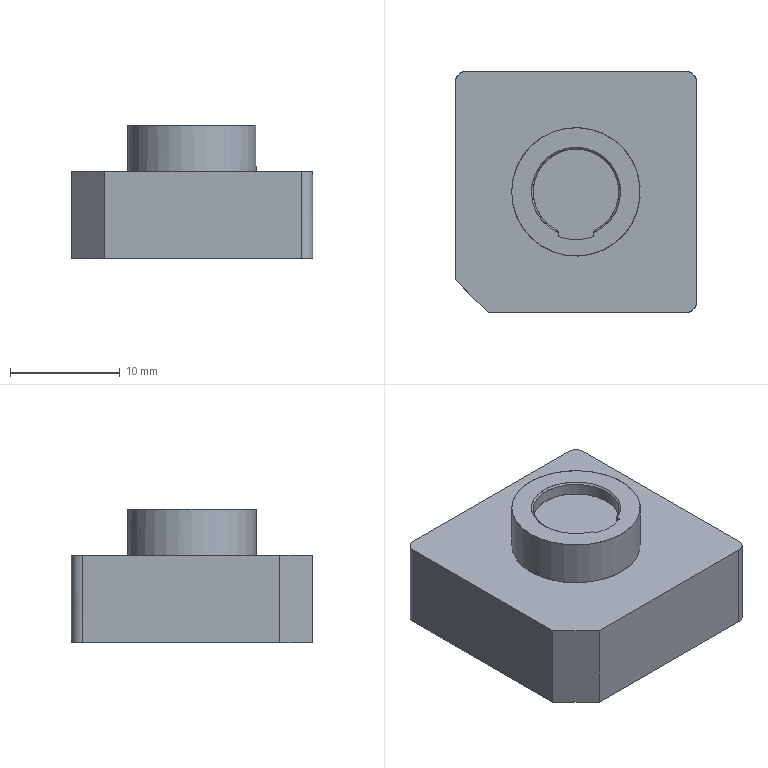NC program | PowerMill | posted by the shop | part box 22 x 22 x 12.219 mm
Lines 1 to 2304 of 55612, first 2083 of 2303 lines:
%
G40 G49 G17 G80
( TOOL ID   D10C_1_1 )
( TOOL DIA. 10. TIP RAD 0 LENGTH 67.68 )
( Z = -.071 )
T1 M6
T15
G91 G28 Z0
G0 G90 G54
M08
S8000 M3
G0 X0 Y0 M8
G43 Z10.2 H1
X13.78 Y13.78
Z1.129
G1 Z-.071 F6000
X-13.78 F10000
Y8.268
X13.78
Y2.756
X-13.78
Y-2.756
X13.78
Y-8.268
X-13.78
Y-13.78
X13.78
X18.78
G0 Z10.2
X0 Y0
Z9.879
X19.055 Y5.589
Z.705
G1 Z-.495 F6000
X18.528 F10000
G3 X13.78 Y.842 I0 J-4.748
G1 Y-12.78
G2 X12.78 Y-13.78 I-1. J0
G1 X-12.78
G2 X-13.78 Y-12.78 I0 J1.
G1 Y12.78
G2 X-12.78 Y13.78 I1. J0
G1 X12.78
G2 X13.78 Y12.78 I0 J-1.
G1 Y.842
X11.106 Y.677
X11.124 Y.387
Y-.387
X11.076 Y-1.16
X10.962 Y-1.934
X10.796 Y-2.707
X10.579 Y-3.48
X10.441 Y-3.857
X9.93 Y-5.027
X9.507 Y-5.801
X8.894 Y-6.698
X8.369 Y-7.348
X7.348 Y-8.369
X6.698 Y-8.894
X5.801 Y-9.507
X5.027 Y-9.93
X3.857 Y-10.441
X3.48 Y-10.579
X2.707 Y-10.796
X1.934 Y-10.962
X1.16 Y-11.076
X.387 Y-11.124
X-.387
X-1.16 Y-11.076
X-1.934 Y-10.962
X-2.707 Y-10.796
X-3.48 Y-10.579
X-3.857 Y-10.441
X-5.027 Y-9.93
X-5.801 Y-9.507
X-6.698 Y-8.894
X-7.348 Y-8.369
X-8.369 Y-7.348
X-8.894 Y-6.698
X-9.507 Y-5.801
X-9.93 Y-5.027
X-10.284 Y-4.254
X-10.579 Y-3.48
X-10.796 Y-2.707
X-10.962 Y-1.934
X-11.076 Y-1.16
X-11.124 Y-.387
Y.387
X-11.076 Y1.16
X-10.962 Y1.934
X-10.796 Y2.707
X-10.579 Y3.48
X-10.441 Y3.857
X-9.93 Y5.027
X-9.507 Y5.801
X-8.894 Y6.698
X-8.369 Y7.348
X-7.348 Y8.369
X-6.698 Y8.894
X-5.801 Y9.507
X-5.027 Y9.93
X-4.254 Y10.284
X-3.48 Y10.579
X-2.707 Y10.796
X-1.934 Y10.962
X-1.16 Y11.076
X-.387 Y11.124
X.387
X1.16 Y11.076
X1.934 Y10.962
X2.707 Y10.796
X3.48 Y10.579
X3.857 Y10.441
X5.027 Y9.93
X5.801 Y9.507
X6.698 Y8.894
X7.348 Y8.369
X8.369 Y7.348
X8.894 Y6.698
X9.507 Y5.801
X9.93 Y5.027
X10.284 Y4.254
X10.579 Y3.48
X10.796 Y2.707
X10.962 Y1.934
X11.076 Y1.16
X11.106 Y.677
X13.78 Y.842
G0 Z3.332
G1 X19.055 Y5.589
G0 Z.332
G1 Z-.868 F6000
X18.528 F10000
G3 X13.78 Y.842 I0 J-4.748
G1 Y-12.78
G2 X12.78 Y-13.78 I-1. J0
G1 X-12.78
G2 X-13.78 Y-12.78 I0 J1.
G1 Y12.78
G2 X-12.78 Y13.78 I1. J0
G1 X12.78
G2 X13.78 Y12.78 I0 J-1.
G1 Y.842
X11.106 Y.677
X11.124 Y.387
Y-.387
X11.076 Y-1.16
X10.962 Y-1.934
X10.796 Y-2.707
X10.579 Y-3.48
X10.441 Y-3.857
X9.93 Y-5.027
X9.507 Y-5.801
X8.894 Y-6.698
X8.369 Y-7.348
X7.348 Y-8.369
X6.698 Y-8.894
X5.801 Y-9.507
X5.027 Y-9.93
X3.857 Y-10.441
X3.48 Y-10.579
X2.707 Y-10.796
X1.934 Y-10.962
X1.16 Y-11.076
X.387 Y-11.124
X-.387
X-1.16 Y-11.076
X-1.934 Y-10.962
X-2.707 Y-10.796
X-3.48 Y-10.579
X-3.857 Y-10.441
X-5.027 Y-9.93
X-5.801 Y-9.507
X-6.698 Y-8.894
X-7.348 Y-8.369
X-8.369 Y-7.348
X-8.894 Y-6.698
X-9.507 Y-5.801
X-9.93 Y-5.027
X-10.284 Y-4.254
X-10.579 Y-3.48
X-10.796 Y-2.707
X-10.962 Y-1.934
X-11.076 Y-1.16
X-11.124 Y-.387
Y.387
X-11.076 Y1.16
X-10.962 Y1.934
X-10.796 Y2.707
X-10.579 Y3.48
X-10.441 Y3.857
X-9.93 Y5.027
X-9.507 Y5.801
X-8.894 Y6.698
X-8.369 Y7.348
X-7.348 Y8.369
X-6.698 Y8.894
X-5.801 Y9.507
X-5.027 Y9.93
X-4.254 Y10.284
X-3.48 Y10.579
X-2.707 Y10.796
X-1.934 Y10.962
X-1.16 Y11.076
X-.387 Y11.124
X.387
X1.16 Y11.076
X1.934 Y10.962
X2.707 Y10.796
X3.48 Y10.579
X3.857 Y10.441
X5.027 Y9.93
X5.801 Y9.507
X6.698 Y8.894
X7.348 Y8.369
X8.369 Y7.348
X8.894 Y6.698
X9.507 Y5.801
X9.93 Y5.027
X10.284 Y4.254
X10.579 Y3.48
X10.796 Y2.707
X10.962 Y1.934
X11.076 Y1.16
X11.106 Y.677
X13.78 Y.842
G0 Z2.958
G1 X19.055 Y5.589
G0 Z-.042
G1 Z-1.242 F6000
X18.528 F10000
G3 X13.78 Y.842 I0 J-4.748
G1 Y-12.78
G2 X12.78 Y-13.78 I-1. J0
G1 X-12.78
G2 X-13.78 Y-12.78 I0 J1.
G1 Y12.78
G2 X-12.78 Y13.78 I1. J0
G1 X12.78
G2 X13.78 Y12.78 I0 J-1.
G1 Y.842
X11.106 Y.677
X11.124 Y.387
Y-.387
X11.076 Y-1.16
X10.962 Y-1.934
X10.796 Y-2.707
X10.579 Y-3.48
X10.441 Y-3.857
X9.93 Y-5.027
X9.507 Y-5.801
X8.894 Y-6.698
X8.369 Y-7.348
X7.348 Y-8.369
X6.698 Y-8.894
X5.801 Y-9.507
X5.027 Y-9.93
X3.857 Y-10.441
X3.48 Y-10.579
X2.707 Y-10.796
X1.934 Y-10.962
X1.16 Y-11.076
X.387 Y-11.124
X-.387
X-1.16 Y-11.076
X-1.934 Y-10.962
X-2.707 Y-10.796
X-3.48 Y-10.579
X-3.857 Y-10.441
X-5.027 Y-9.93
X-5.801 Y-9.507
X-6.698 Y-8.894
X-7.348 Y-8.369
X-8.369 Y-7.348
X-8.894 Y-6.698
X-9.507 Y-5.801
X-9.93 Y-5.027
X-10.284 Y-4.254
X-10.579 Y-3.48
X-10.796 Y-2.707
X-10.962 Y-1.934
X-11.076 Y-1.16
X-11.124 Y-.387
Y.387
X-11.076 Y1.16
X-10.962 Y1.934
X-10.796 Y2.707
X-10.579 Y3.48
X-10.441 Y3.857
X-9.93 Y5.027
X-9.507 Y5.801
X-8.894 Y6.698
X-8.369 Y7.348
X-7.348 Y8.369
X-6.698 Y8.894
X-5.801 Y9.507
X-5.027 Y9.93
X-4.254 Y10.284
X-3.48 Y10.579
X-2.707 Y10.796
X-1.934 Y10.962
X-1.16 Y11.076
X-.387 Y11.124
X.387
X1.16 Y11.076
X1.934 Y10.962
X2.707 Y10.796
X3.48 Y10.579
X3.857 Y10.441
X5.027 Y9.93
X5.801 Y9.507
X6.698 Y8.894
X7.348 Y8.369
X8.369 Y7.348
X8.894 Y6.698
X9.507 Y5.801
X9.93 Y5.027
X10.284 Y4.254
X10.579 Y3.48
X10.796 Y2.707
X10.962 Y1.934
X11.076 Y1.16
X11.106 Y.677
X13.78 Y.842
G0 Z2.585
G1 X19.055 Y5.589
G0 Z-.415
G1 Z-1.615 F6000
X18.528 F10000
G3 X13.78 Y.842 I0 J-4.748
G1 Y-12.78
G2 X12.78 Y-13.78 I-1. J0
G1 X-12.78
G2 X-13.78 Y-12.78 I0 J1.
G1 Y12.78
G2 X-12.78 Y13.78 I1. J0
G1 X12.78
G2 X13.78 Y12.78 I0 J-1.
G1 Y.842
X11.106 Y.677
X11.124 Y.387
Y-.387
X11.076 Y-1.16
X10.962 Y-1.934
X10.796 Y-2.707
X10.579 Y-3.48
X10.441 Y-3.857
X9.93 Y-5.027
X9.507 Y-5.801
X8.894 Y-6.698
X8.369 Y-7.348
X7.348 Y-8.369
X6.698 Y-8.894
X5.801 Y-9.507
X5.027 Y-9.93
X3.857 Y-10.441
X3.48 Y-10.579
X2.707 Y-10.796
X1.934 Y-10.962
X1.16 Y-11.076
X.387 Y-11.124
X-.387
X-1.16 Y-11.076
X-1.934 Y-10.962
X-2.707 Y-10.796
X-3.48 Y-10.579
X-3.857 Y-10.441
X-5.027 Y-9.93
X-5.801 Y-9.507
X-6.698 Y-8.894
X-7.348 Y-8.369
X-8.369 Y-7.348
X-8.894 Y-6.698
X-9.507 Y-5.801
X-9.93 Y-5.027
X-10.284 Y-4.254
X-10.579 Y-3.48
X-10.796 Y-2.707
X-10.962 Y-1.934
X-11.076 Y-1.16
X-11.124 Y-.387
Y.387
X-11.076 Y1.16
X-10.962 Y1.934
X-10.796 Y2.707
X-10.579 Y3.48
X-10.441 Y3.857
X-9.93 Y5.027
X-9.507 Y5.801
X-8.894 Y6.698
X-8.369 Y7.348
X-7.348 Y8.369
X-6.698 Y8.894
X-5.801 Y9.507
X-5.027 Y9.93
X-4.254 Y10.284
X-3.48 Y10.579
X-2.707 Y10.796
X-1.934 Y10.962
X-1.16 Y11.076
X-.387 Y11.124
X.387
X1.16 Y11.076
X1.934 Y10.962
X2.707 Y10.796
X3.48 Y10.579
X3.857 Y10.441
X5.027 Y9.93
X5.801 Y9.507
X6.698 Y8.894
X7.348 Y8.369
X8.369 Y7.348
X8.894 Y6.698
X9.507 Y5.801
X9.93 Y5.027
X10.284 Y4.254
X10.579 Y3.48
X10.796 Y2.707
X10.962 Y1.934
X11.076 Y1.16
X11.106 Y.677
X13.78 Y.842
G0 Z2.211
G1 X19.055 Y5.589
G0 Z-.789
G1 Z-1.989 F6000
X18.528 F10000
G3 X13.78 Y.842 I0 J-4.748
G1 Y-12.78
G2 X12.78 Y-13.78 I-1. J0
G1 X-12.78
G2 X-13.78 Y-12.78 I0 J1.
G1 Y12.78
G2 X-12.78 Y13.78 I1. J0
G1 X12.78
G2 X13.78 Y12.78 I0 J-1.
G1 Y.842
X11.106 Y.677
X11.124 Y.387
Y-.387
X11.076 Y-1.16
X10.962 Y-1.934
X10.796 Y-2.707
X10.579 Y-3.48
X10.441 Y-3.857
X9.93 Y-5.027
X9.507 Y-5.801
X8.894 Y-6.698
X8.369 Y-7.348
X7.348 Y-8.369
X6.698 Y-8.894
X5.801 Y-9.507
X5.027 Y-9.93
X3.857 Y-10.441
X3.48 Y-10.579
X2.707 Y-10.796
X1.934 Y-10.962
X1.16 Y-11.076
X.387 Y-11.124
X-.387
X-1.16 Y-11.076
X-1.934 Y-10.962
X-2.707 Y-10.796
X-3.48 Y-10.579
X-3.857 Y-10.441
X-5.027 Y-9.93
X-5.801 Y-9.507
X-6.698 Y-8.894
X-7.348 Y-8.369
X-8.369 Y-7.348
X-8.894 Y-6.698
X-9.507 Y-5.801
X-9.93 Y-5.027
X-10.284 Y-4.254
X-10.579 Y-3.48
X-10.796 Y-2.707
X-10.962 Y-1.934
X-11.076 Y-1.16
X-11.124 Y-.387
Y.387
X-11.076 Y1.16
X-10.962 Y1.934
X-10.796 Y2.707
X-10.579 Y3.48
X-10.441 Y3.857
X-9.93 Y5.027
X-9.507 Y5.801
X-8.894 Y6.698
X-8.369 Y7.348
X-7.348 Y8.369
X-6.698 Y8.894
X-5.801 Y9.507
X-5.027 Y9.93
X-4.254 Y10.284
X-3.48 Y10.579
X-2.707 Y10.796
X-1.934 Y10.962
X-1.16 Y11.076
X-.387 Y11.124
X.387
X1.16 Y11.076
X1.934 Y10.962
X2.707 Y10.796
X3.48 Y10.579
X3.857 Y10.441
X5.027 Y9.93
X5.801 Y9.507
X6.698 Y8.894
X7.348 Y8.369
X8.369 Y7.348
X8.894 Y6.698
X9.507 Y5.801
X9.93 Y5.027
X10.284 Y4.254
X10.579 Y3.48
X10.796 Y2.707
X10.962 Y1.934
X11.076 Y1.16
X11.106 Y.677
X13.78 Y.842
G0 Z1.838
G1 X19.055 Y5.589
G0 Z-1.162
G1 Z-2.362 F6000
X18.528 F10000
G3 X13.78 Y.842 I0 J-4.748
G1 Y-12.78
G2 X12.78 Y-13.78 I-1. J0
G1 X-12.78
G2 X-13.78 Y-12.78 I0 J1.
G1 Y12.78
G2 X-12.78 Y13.78 I1. J0
G1 X12.78
G2 X13.78 Y12.78 I0 J-1.
G1 Y.842
X11.106 Y.677
X11.124 Y.387
Y-.387
X11.076 Y-1.16
X10.962 Y-1.934
X10.796 Y-2.707
X10.579 Y-3.48
X10.441 Y-3.857
X9.93 Y-5.027
X9.507 Y-5.801
X8.894 Y-6.698
X8.369 Y-7.348
X7.348 Y-8.369
X6.698 Y-8.894
X5.801 Y-9.507
X5.027 Y-9.93
X3.857 Y-10.441
X3.48 Y-10.579
X2.707 Y-10.796
X1.934 Y-10.962
X1.16 Y-11.076
X.387 Y-11.124
X-.387
X-1.16 Y-11.076
X-1.934 Y-10.962
X-2.707 Y-10.796
X-3.48 Y-10.579
X-3.857 Y-10.441
X-5.027 Y-9.93
X-5.801 Y-9.507
X-6.698 Y-8.894
X-7.348 Y-8.369
X-8.369 Y-7.348
X-8.894 Y-6.698
X-9.507 Y-5.801
X-9.93 Y-5.027
X-10.284 Y-4.254
X-10.579 Y-3.48
X-10.796 Y-2.707
X-10.962 Y-1.934
X-11.076 Y-1.16
X-11.124 Y-.387
Y.387
X-11.076 Y1.16
X-10.962 Y1.934
X-10.796 Y2.707
X-10.579 Y3.48
X-10.441 Y3.857
X-9.93 Y5.027
X-9.507 Y5.801
X-8.894 Y6.698
X-8.369 Y7.348
X-7.348 Y8.369
X-6.698 Y8.894
X-5.801 Y9.507
X-5.027 Y9.93
X-4.254 Y10.284
X-3.48 Y10.579
X-2.707 Y10.796
X-1.934 Y10.962
X-1.16 Y11.077
X-.387 Y11.124
X.387
X1.16 Y11.077
X1.934 Y10.962
X2.707 Y10.796
X3.48 Y10.579
X3.857 Y10.441
X5.027 Y9.93
X5.801 Y9.507
X6.698 Y8.894
X7.348 Y8.369
X8.369 Y7.348
X8.894 Y6.698
X9.507 Y5.801
X9.93 Y5.027
X10.284 Y4.254
X10.579 Y3.48
X10.796 Y2.707
X10.962 Y1.934
X11.076 Y1.16
X11.106 Y.677
X13.78 Y.842
G0 Z1.464
G1 X19.055 Y5.589
G0 Z-1.536
G1 Z-2.736 F6000
X18.528 F10000
G3 X13.78 Y.842 I0 J-4.748
G1 Y-12.78
G2 X12.78 Y-13.78 I-1. J0
G1 X-12.78
G2 X-13.78 Y-12.78 I0 J1.
G1 Y12.78
G2 X-12.78 Y13.78 I1. J0
G1 X12.78
G2 X13.78 Y12.78 I0 J-1.
G1 Y.842
X11.106 Y.677
X11.124 Y.387
Y-.387
X11.077 Y-1.16
X10.962 Y-1.934
X10.796 Y-2.707
X10.579 Y-3.48
X10.441 Y-3.857
X9.93 Y-5.027
X9.507 Y-5.801
X8.894 Y-6.698
X8.369 Y-7.348
X7.348 Y-8.369
X6.698 Y-8.894
X5.801 Y-9.507
X5.027 Y-9.93
X3.857 Y-10.441
X3.48 Y-10.579
X2.707 Y-10.796
X1.934 Y-10.962
X1.16 Y-11.077
X.387 Y-11.124
X-.387
X-1.16 Y-11.077
X-1.934 Y-10.962
X-2.707 Y-10.796
X-3.48 Y-10.579
X-3.857 Y-10.441
X-5.027 Y-9.93
X-5.801 Y-9.507
X-6.698 Y-8.894
X-7.348 Y-8.369
X-8.369 Y-7.348
X-8.894 Y-6.698
X-9.507 Y-5.801
X-9.93 Y-5.027
X-10.284 Y-4.254
X-10.579 Y-3.48
X-10.796 Y-2.707
X-10.962 Y-1.934
X-11.077 Y-1.16
X-11.124 Y-.387
Y.387
X-11.077 Y1.16
X-10.962 Y1.934
X-10.796 Y2.707
X-10.579 Y3.48
X-10.441 Y3.857
X-9.93 Y5.027
X-9.507 Y5.801
X-8.894 Y6.698
X-8.369 Y7.348
X-7.348 Y8.369
X-6.698 Y8.894
X-5.801 Y9.507
X-5.027 Y9.93
X-4.254 Y10.284
X-3.48 Y10.579
X-2.707 Y10.796
X-1.934 Y10.962
X-1.16 Y11.077
X-.387 Y11.124
X.387
X1.16 Y11.077
X1.934 Y10.962
X2.707 Y10.796
X3.48 Y10.579
X3.857 Y10.441
X5.027 Y9.93
X5.801 Y9.507
X6.698 Y8.894
X7.348 Y8.369
X8.369 Y7.348
X8.894 Y6.698
X9.507 Y5.801
X9.93 Y5.027
X10.284 Y4.254
X10.579 Y3.48
X10.796 Y2.707
X10.962 Y1.934
X11.077 Y1.16
X11.106 Y.677
X13.78 Y.842
G0 Z1.091
G1 X19.055 Y5.589
G0 Z-1.909
G1 Z-3.109 F6000
X18.528 F10000
G3 X13.78 Y.842 I0 J-4.748
G1 Y-12.78
G2 X12.78 Y-13.78 I-1. J0
G1 X-12.78
G2 X-13.78 Y-12.78 I0 J1.
G1 Y12.78
G2 X-12.78 Y13.78 I1. J0
G1 X12.78
G2 X13.78 Y12.78 I0 J-1.
G1 Y.842
X11.106 Y.677
X11.124 Y.387
Y-.387
X11.077 Y-1.16
X10.962 Y-1.934
X10.796 Y-2.707
X10.579 Y-3.48
X10.441 Y-3.857
X9.93 Y-5.027
X9.507 Y-5.801
X8.894 Y-6.698
X8.369 Y-7.348
X7.348 Y-8.369
X6.698 Y-8.894
X5.801 Y-9.507
X5.027 Y-9.93
X3.857 Y-10.441
X3.48 Y-10.579
X2.707 Y-10.796
X1.934 Y-10.962
X1.16 Y-11.077
X.387 Y-11.124
X-.387
X-1.16 Y-11.077
X-1.934 Y-10.962
X-2.707 Y-10.796
X-3.48 Y-10.579
X-3.857 Y-10.441
X-5.027 Y-9.93
X-5.801 Y-9.507
X-6.698 Y-8.894
X-7.348 Y-8.369
X-8.369 Y-7.348
X-8.894 Y-6.698
X-9.507 Y-5.801
X-9.93 Y-5.027
X-10.284 Y-4.254
X-10.579 Y-3.48
X-10.796 Y-2.707
X-10.962 Y-1.934
X-11.077 Y-1.16
X-11.124 Y-.387
Y.387
X-11.077 Y1.16
X-10.962 Y1.934
X-10.796 Y2.707
X-10.579 Y3.48
X-10.441 Y3.857
X-9.93 Y5.027
X-9.507 Y5.801
X-8.894 Y6.698
X-8.369 Y7.348
X-7.348 Y8.369
X-6.698 Y8.894
X-5.801 Y9.507
X-5.027 Y9.93
X-4.254 Y10.284
X-3.48 Y10.579
X-2.707 Y10.796
X-1.934 Y10.962
X-1.16 Y11.077
X-.387 Y11.124
X.387
X1.16 Y11.077
X1.934 Y10.962
X2.707 Y10.796
X3.48 Y10.579
X3.857 Y10.441
X5.027 Y9.93
X5.801 Y9.507
X6.698 Y8.894
X7.348 Y8.369
X8.369 Y7.348
X8.894 Y6.698
X9.507 Y5.801
X9.93 Y5.027
X10.284 Y4.254
X10.579 Y3.48
X10.796 Y2.707
X10.962 Y1.934
X11.077 Y1.16
X11.106 Y.677
X13.78 Y.842
G0 Z.717
G1 X19.055 Y5.589
G0 Z-2.283
G1 Z-3.483 F6000
X18.528 F10000
G3 X13.78 Y.842 I0 J-4.748
G1 Y-12.78
G2 X12.78 Y-13.78 I-1. J0
G1 X-12.78
G2 X-13.78 Y-12.78 I0 J1.
G1 Y12.78
G2 X-12.78 Y13.78 I1. J0
G1 X12.78
G2 X13.78 Y12.78 I0 J-1.
G1 Y.842
X11.106 Y.677
X11.124 Y.387
Y-.387
X11.077 Y-1.16
X10.962 Y-1.934
X10.796 Y-2.707
X10.579 Y-3.48
X10.441 Y-3.857
X9.93 Y-5.027
X9.507 Y-5.801
X8.894 Y-6.698
X8.369 Y-7.348
X7.348 Y-8.369
X6.698 Y-8.894
X5.801 Y-9.507
X5.027 Y-9.93
X3.857 Y-10.441
X3.48 Y-10.579
X2.707 Y-10.796
X1.934 Y-10.962
X1.16 Y-11.077
X.387 Y-11.124
X-.387
X-1.16 Y-11.077
X-1.934 Y-10.962
X-2.707 Y-10.796
X-3.48 Y-10.579
X-3.857 Y-10.441
X-5.027 Y-9.93
X-5.801 Y-9.507
X-6.698 Y-8.894
X-7.348 Y-8.369
X-8.369 Y-7.348
X-8.894 Y-6.698
X-9.507 Y-5.801
X-9.93 Y-5.027
X-10.284 Y-4.254
X-10.579 Y-3.48
X-10.796 Y-2.707
X-10.962 Y-1.934
X-11.077 Y-1.16
X-11.124 Y-.387
Y.387
X-11.077 Y1.16
X-10.962 Y1.934
X-10.796 Y2.707
X-10.579 Y3.48
X-10.441 Y3.857
X-9.93 Y5.027
X-9.507 Y5.801
X-8.894 Y6.698
X-8.369 Y7.348
X-7.348 Y8.369
X-6.698 Y8.894
X-5.801 Y9.507
X-5.027 Y9.93
X-4.254 Y10.284
X-3.48 Y10.579
X-2.707 Y10.796
X-1.934 Y10.962
X-1.16 Y11.077
X-.387 Y11.124
X.387
X1.16 Y11.077
X1.934 Y10.962
X2.707 Y10.796
X3.48 Y10.579
X3.857 Y10.441
X5.027 Y9.93
X5.801 Y9.507
X6.698 Y8.894
X7.348 Y8.369
X8.369 Y7.348
X8.894 Y6.698
X9.507 Y5.801
X9.93 Y5.027
X10.284 Y4.254
X10.579 Y3.48
X10.796 Y2.707
X10.962 Y1.934
X11.077 Y1.16
X11.106 Y.677
X13.78 Y.842
G0 Z.344
G1 X19.055 Y5.589
G0 Z-2.656
G1 Z-3.856 F6000
X18.528 F10000
G3 X13.78 Y.842 I0 J-4.748
G1 Y-12.78
G2 X12.78 Y-13.78 I-1. J0
G1 X-12.78
G2 X-13.78 Y-12.78 I0 J1.
G1 Y12.78
G2 X-12.78 Y13.78 I1. J0
G1 X12.78
G2 X13.78 Y12.78 I0 J-1.
G1 Y.842
X11.106 Y.677
X11.124 Y.387
Y-.387
X11.077 Y-1.16
X10.962 Y-1.934
X10.796 Y-2.707
X10.579 Y-3.48
X10.441 Y-3.857
X9.93 Y-5.027
X9.507 Y-5.801
X8.894 Y-6.698
X8.369 Y-7.348
X7.348 Y-8.369
X6.698 Y-8.894
X5.801 Y-9.507
X5.027 Y-9.93
X3.857 Y-10.441
X3.48 Y-10.579
X2.707 Y-10.796
X1.934 Y-10.962
X1.16 Y-11.077
X.387 Y-11.124
X-.387
X-1.16 Y-11.077
X-1.934 Y-10.962
X-2.707 Y-10.796
X-3.48 Y-10.579
X-3.857 Y-10.441
X-5.027 Y-9.93
X-5.801 Y-9.507
X-6.698 Y-8.894
X-7.348 Y-8.369
X-8.369 Y-7.348
X-8.894 Y-6.698
X-9.507 Y-5.801
X-9.93 Y-5.027
X-10.284 Y-4.254
X-10.579 Y-3.48
X-10.796 Y-2.707
X-10.962 Y-1.934
X-11.077 Y-1.16
X-11.124 Y-.387
Y.387
X-11.077 Y1.16
X-10.962 Y1.934
X-10.796 Y2.707
X-10.579 Y3.48
X-10.441 Y3.857
X-9.93 Y5.027
X-9.507 Y5.801
X-8.894 Y6.698
X-8.369 Y7.348
X-7.348 Y8.369
X-6.698 Y8.894
X-5.801 Y9.507
X-5.027 Y9.93
X-4.254 Y10.284
X-3.48 Y10.579
X-2.707 Y10.796
X-1.934 Y10.962
X-1.16 Y11.077
X-.387 Y11.124
X.387
X1.16 Y11.077
X1.934 Y10.962
X2.707 Y10.796
X3.48 Y10.579
X3.857 Y10.441
X5.027 Y9.93
X5.801 Y9.507
X6.698 Y8.894
X7.348 Y8.369
X8.369 Y7.348
X8.894 Y6.698
X9.507 Y5.801
X9.93 Y5.027
X10.284 Y4.254
X10.579 Y3.48
X10.796 Y2.707
X10.962 Y1.934
X11.077 Y1.16
X11.106 Y.677
X13.78 Y.842
G0 Z-.03
G1 X19.055 Y5.589
G0 Z-3.03
G1 Z-4.23 F6000
X18.528 F10000
G3 X13.78 Y.842 I0 J-4.748
G1 Y-12.78
G2 X12.78 Y-13.78 I-1. J0
G1 X-12.78
G2 X-13.78 Y-12.78 I0 J1.
G1 Y12.78
G2 X-12.78 Y13.78 I1. J0
G1 X12.78
G2 X13.78 Y12.78 I0 J-1.
G1 Y.842
X11.106 Y.677
X11.124 Y.387
Y-.387
X11.077 Y-1.16
X10.962 Y-1.934
X10.796 Y-2.707
X10.579 Y-3.48
X10.441 Y-3.857
X9.93 Y-5.027
X9.507 Y-5.801
X8.894 Y-6.698
X8.369 Y-7.348
X7.348 Y-8.369
X6.698 Y-8.894
X5.801 Y-9.507
X5.027 Y-9.93
X3.857 Y-10.441
X3.48 Y-10.579
X2.707 Y-10.796
X1.934 Y-10.962
X1.16 Y-11.077
X.387 Y-11.124
X-.387
X-1.16 Y-11.077
X-1.934 Y-10.962
X-2.707 Y-10.796
X-3.48 Y-10.579
X-3.857 Y-10.441
X-5.027 Y-9.93
X-5.801 Y-9.507
X-6.698 Y-8.894
X-7.348 Y-8.369
X-8.369 Y-7.348
X-8.894 Y-6.698
X-9.507 Y-5.801
X-9.93 Y-5.027
X-10.284 Y-4.254
X-10.579 Y-3.48
X-10.796 Y-2.707
X-10.962 Y-1.934
X-11.077 Y-1.16
X-11.124 Y-.387
Y.387
X-11.077 Y1.16
X-10.962 Y1.934
X-10.796 Y2.707
X-10.579 Y3.48
X-10.441 Y3.857
X-9.93 Y5.027
X-9.507 Y5.801
X-8.894 Y6.698
X-8.369 Y7.348
X-7.348 Y8.369
X-6.698 Y8.894
X-5.801 Y9.507
X-5.027 Y9.93
X-4.254 Y10.284
X-3.48 Y10.579
X-2.707 Y10.796
X-1.934 Y10.962
X-1.16 Y11.077
X-.387 Y11.124
X.387
X1.16 Y11.077
X1.934 Y10.962
X2.707 Y10.796
X3.48 Y10.579
X3.857 Y10.441
X5.027 Y9.93
X5.801 Y9.507
X6.698 Y8.894
X7.348 Y8.369
X8.369 Y7.348
X8.894 Y6.698
X9.507 Y5.801
X9.93 Y5.027
X10.284 Y4.254
X10.579 Y3.48
X10.796 Y2.707
X10.962 Y1.934
X11.077 Y1.16
X11.106 Y.677
X13.78 Y.842
G0 Z9.879
X0 Y0
Z9.799
X15.059 Y-20.955
Z-3.408
G1 Z-4.608 F6000
G3 X12.629 Y-15.469 I-1.215 J2.743 F10000
G1 X12.375 Y-15.581
X11.601 Y-15.855
X10.828 Y-16.006
X10.055 Y-16.07
X-7.734
X-8.508 Y-16.044
X-9.281 Y-15.905
X-10.055 Y-15.635
X-10.395 Y-15.469
X-10.828 Y-15.208
X-11.471 Y-14.695
X-14.695 Y-11.471
X-15.208 Y-10.828
X-15.469 Y-10.395
X-15.635 Y-10.055
X-15.905 Y-9.281
X-16.044 Y-8.508
X-16.07 Y-7.734
Y10.055
X-16.006 Y10.828
X-15.855 Y11.601
X-15.581 Y12.375
X-15.189 Y13.148
X-14.629 Y13.922
X-13.844 Y14.695
X-13.148 Y15.189
X-12.375 Y15.581
X-11.601 Y15.855
X-10.828 Y16.006
X-10.055 Y16.07
X10.055
X10.828 Y16.006
X11.601 Y15.855
X12.375 Y15.581
X13.148 Y15.189
X13.922 Y14.629
X14.695 Y13.844
X15.189 Y13.148
X15.581 Y12.375
X15.855 Y11.601
X16.006 Y10.828
X16.07 Y10.055
Y-10.055
X16.006 Y-10.828
X15.855 Y-11.601
X15.581 Y-12.375
X15.189 Y-13.148
X14.629 Y-13.922
X13.844 Y-14.695
X13.148 Y-15.189
X12.629 Y-15.469
X12.375 Y-15.581 Z-4.609
X11.601 Y-15.855 Z-4.612
X10.828 Y-16.006 Z-4.614
X10.055 Y-16.07 Z-4.617
X-7.734 Z-4.676
X-8.52 Y-16.043 Z-4.679
X-9.293 Y-15.902 Z-4.681
X-10.06 Y-15.633 Z-4.684
X-10.395 Y-15.469 Z-4.685
X-10.839 Y-15.201 Z-4.687
X-11.471 Y-14.695 Z-4.69
X-14.695 Y-11.471 Z-4.705
X-15.208 Y-10.828 Z-4.708
X-15.469 Y-10.395 Z-4.709
X-15.635 Y-10.055 Z-4.71
X-15.905 Y-9.281 Z-4.713
X-16.045 Y-8.508 Z-4.716
X-16.07 Y-7.734 Z-4.718
Y10.067 Z-4.778
X-16.005 Y10.84 Z-4.78
X-15.851 Y11.614 Z-4.783
X-15.579 Y12.379 Z-4.785
X-15.182 Y13.16 Z-4.788
X-14.618 Y13.933 Z-4.792
X-14.259 Y14.325 Z-4.793
X-13.864 Y14.679 Z-4.795
X-13.148 Y15.189 Z-4.798
X-12.375 Y15.581 Z-4.801
X-11.601 Y15.855 Z-4.804
X-10.828 Y16.006 Z-4.806
X-10.055 Y16.07 Z-4.809
X10.055 Z-4.876
X10.84 Y16.005 Z-4.878
X11.614 Y15.851 Z-4.881
X12.379 Y15.579 Z-4.884
X13.16 Y15.182 Z-4.886
X13.933 Y14.618 Z-4.89
X14.325 Y14.259 Z-4.891
X14.679 Y13.864 Z-4.893
X15.189 Y13.148 Z-4.896
X15.581 Y12.375 Z-4.899
X15.855 Y11.601 Z-4.902
X16.006 Y10.828 Z-4.904
X16.07 Y10.055 Z-4.907
Y-10.055 Z-4.974
X16.005 Y-10.84 Z-4.976
X15.851 Y-11.614 Z-4.979
X15.579 Y-12.379 Z-4.982
X15.182 Y-13.16 Z-4.985
X14.618 Y-13.933 Z-4.988
X14.259 Y-14.325 Z-4.99
X13.864 Y-14.679 Z-4.991
X13.148 Y-15.189 Z-4.994
X12.629 Y-15.469 Z-4.996
X12.375 Y-15.581 Z-4.997
X11.601 Y-15.855 Z-5.
X10.828 Y-16.006 Z-5.002
X10.055 Y-16.07 Z-5.005
X-7.734 Z-5.064
X-8.52 Y-16.043 Z-5.067
X-9.293 Y-15.902 Z-5.069
X-10.06 Y-15.633 Z-5.072
X-10.395 Y-15.469 Z-5.073
X-10.839 Y-15.201 Z-5.075
X-11.471 Y-14.695 Z-5.078
X-14.695 Y-11.471 Z-5.093
X-15.208 Y-10.828 Z-5.096
X-15.469 Y-10.395 Z-5.097
X-15.635 Y-10.055 Z-5.099
X-15.905 Y-9.281 Z-5.101
X-16.045 Y-8.508 Z-5.104
X-16.07 Y-7.734 Z-5.106
Y10.055 Z-5.166
X-16.005 Y10.84 Z-5.168
X-15.851 Y11.614 Z-5.171
X-15.579 Y12.379 Z-5.174
X-15.182 Y13.16 Z-5.176
X-14.618 Y13.933 Z-5.18
X-14.259 Y14.325 Z-5.181
X-13.864 Y14.679 Z-5.183
X-13.148 Y15.189 Z-5.186
X-12.375 Y15.581 Z-5.189
X-11.601 Y15.855 Z-5.192
X-10.828 Y16.006 Z-5.194
X-10.055 Y16.07 Z-5.197
X10.055 Z-5.264
X10.84 Y16.005 Z-5.266
X11.614 Y15.851 Z-5.269
X12.379 Y15.579 Z-5.272
X13.16 Y15.182 Z-5.275
X13.933 Y14.618 Z-5.278
X14.325 Y14.259 Z-5.28
X14.679 Y13.864 Z-5.281
X15.189 Y13.148 Z-5.284
X15.581 Y12.375 Z-5.287
X15.855 Y11.601 Z-5.29
X16.006 Y10.828 Z-5.292
X16.07 Y10.055 Z-5.295
Y-10.055 Z-5.362
X16.005 Y-10.84 Z-5.364
X15.851 Y-11.614 Z-5.367
X15.579 Y-12.379 Z-5.37
X15.182 Y-13.16 Z-5.373
X14.618 Y-13.933 Z-5.376
X14.259 Y-14.325 Z-5.378
X13.864 Y-14.679 Z-5.379
X13.148 Y-15.189 Z-5.382
X12.629 Y-15.469 Z-5.384
X12.363 Y-15.586 Z-5.385
X11.601 Y-15.855 Z-5.388
X10.828 Y-16.006 Z-5.391
X10.055 Y-16.07 Z-5.393
X-7.734 Z-5.452
X-8.52 Y-16.043 Z-5.455
X-9.293 Y-15.902 Z-5.457
X-10.06 Y-15.633 Z-5.46
X-10.395 Y-15.469 Z-5.461
X-10.839 Y-15.201 Z-5.463
X-11.471 Y-14.695 Z-5.466
X-14.695 Y-11.471 Z-5.481
X-15.208 Y-10.828 Z-5.484
X-15.469 Y-10.395 Z-5.485
X-15.635 Y-10.055 Z-5.487
X-15.905 Y-9.281 Z-5.489
X-16.045 Y-8.508 Z-5.492
X-16.07 Y-7.734 Z-5.495
Y10.055 Z-5.554
X-16.005 Y10.84 Z-5.556
X-15.851 Y11.614 Z-5.559
X-15.579 Y12.379 Z-5.562
X-15.182 Y13.16 Z-5.565
X-14.618 Y13.933 Z-5.568
X-14.259 Y14.325 Z-5.569
X-13.864 Y14.679 Z-5.571
X-13.148 Y15.189 Z-5.574
X-12.375 Y15.581 Z-5.577
X-11.601 Y15.855 Z-5.58
X-10.828 Y16.006 Z-5.582
X-10.055 Y16.07 Z-5.585
X10.055 Z-5.652
X10.84 Y16.005 Z-5.654
X11.614 Y15.851 Z-5.657
X12.379 Y15.579 Z-5.66
X13.16 Y15.182 Z-5.663
X13.933 Y14.618 Z-5.666
X14.325 Y14.259 Z-5.668
X14.679 Y13.864 Z-5.669
X15.189 Y13.148 Z-5.672
X15.581 Y12.375 Z-5.675
X15.855 Y11.601 Z-5.678
X16.006 Y10.828 Z-5.681
X16.07 Y10.055 Z-5.683
Y-10.055 Z-5.75
X16.005 Y-10.84 Z-5.753
X15.851 Y-11.614 Z-5.755
X15.579 Y-12.379 Z-5.758
X15.182 Y-13.16 Z-5.761
X14.618 Y-13.933 Z-5.764
X14.259 Y-14.325 Z-5.766
X13.864 Y-14.679 Z-5.767
X13.148 Y-15.189 Z-5.77
X12.629 Y-15.469 Z-5.772
X12.375 Y-15.581 Z-5.773
X11.601 Y-15.855 Z-5.776
X10.828 Y-16.006 Z-5.779
X10.055 Y-16.07 Z-5.781
X-7.734 Z-5.84
X-8.52 Y-16.043 Z-5.843
X-9.293 Y-15.902 Z-5.846
X-10.06 Y-15.633 Z-5.848
X-10.395 Y-15.469 Z-5.85
X-10.839 Y-15.201 Z-5.851
X-11.471 Y-14.695 Z-5.854
X-14.695 Y-11.471 Z-5.869
X-15.208 Y-10.828 Z-5.872
X-15.471 Y-10.39 Z-5.874
X-15.635 Y-10.055 Z-5.875
X-15.905 Y-9.281 Z-5.877
X-16.045 Y-8.508 Z-5.88
X-16.07 Y-7.734 Z-5.883
Y10.067 Z-5.942
X-16.005 Y10.84 Z-5.944
X-15.851 Y11.614 Z-5.947
X-15.579 Y12.379 Z-5.95
X-15.182 Y13.16 Z-5.953
X-14.618 Y13.933 Z-5.956
X-14.259 Y14.325 Z-5.958
X-13.864 Y14.679 Z-5.959
X-13.148 Y15.189 Z-5.962
X-12.375 Y15.581 Z-5.965
X-11.601 Y15.855 Z-5.968
X-10.828 Y16.006 Z-5.97
X-10.055 Y16.07 Z-5.973
X10.055 Z-6.04
X10.84 Y16.005 Z-6.043
X11.614 Y15.851 Z-6.045
X12.379 Y15.579 Z-6.048
X13.16 Y15.182 Z-6.051
X13.933 Y14.618 Z-6.054
X14.325 Y14.259 Z-6.056
X14.679 Y13.864 Z-6.057
X15.189 Y13.148 Z-6.06
X15.581 Y12.375 Z-6.063
X15.855 Y11.601 Z-6.066
X16.006 Y10.828 Z-6.069
X16.07 Y10.055 Z-6.071
Y-10.055 Z-6.138
X16.005 Y-10.84 Z-6.141
X15.851 Y-11.614 Z-6.143
X15.579 Y-12.379 Z-6.146
X15.182 Y-13.16 Z-6.149
X14.618 Y-13.933 Z-6.152
X14.259 Y-14.325 Z-6.154
X13.864 Y-14.679 Z-6.156
X13.148 Y-15.189 Z-6.159
X12.629 Y-15.469 Z-6.16
X12.375 Y-15.581 Z-6.161
X11.601 Y-15.855 Z-6.164
X10.828 Y-16.006 Z-6.167
X10.055 Y-16.07 Z-6.169
X-7.734 Z-6.228
X-8.52 Y-16.043 Z-6.231
X-9.293 Y-15.902 Z-6.234
X-10.06 Y-15.633 Z-6.236
X-10.395 Y-15.469 Z-6.238
X-10.839 Y-15.201 Z-6.239
X-11.471 Y-14.695 Z-6.242
X-14.695 Y-11.471 Z-6.257
X-15.208 Y-10.828 Z-6.26
X-15.469 Y-10.395 Z-6.262
X-15.635 Y-10.055 Z-6.263
X-15.905 Y-9.281 Z-6.266
X-16.045 Y-8.508 Z-6.268
X-16.07 Y-7.734 Z-6.271
Y10.055 Z-6.33
X-16.005 Y10.84 Z-6.333
X-15.851 Y11.614 Z-6.335
X-15.579 Y12.379 Z-6.338
X-15.182 Y13.16 Z-6.341
X-14.618 Y13.933 Z-6.344
X-14.259 Y14.325 Z-6.346
X-13.864 Y14.679 Z-6.347
X-13.148 Y15.189 Z-6.35
X-12.375 Y15.581 Z-6.353
X-11.601 Y15.855 Z-6.356
X-10.828 Y16.006 Z-6.359
X-10.055 Y16.07 Z-6.361
X10.055 Z-6.428
X10.84 Y16.005 Z-6.431
X11.614 Y15.851 Z-6.433
X12.379 Y15.579 Z-6.436
X13.16 Y15.182 Z-6.439
X13.933 Y14.618 Z-6.442
X14.325 Y14.259 Z-6.444
X14.679 Y13.864 Z-6.446
X15.189 Y13.148 Z-6.448
X15.581 Y12.375 Z-6.451
X15.855 Y11.601 Z-6.454
X16.006 Y10.828 Z-6.457
X16.07 Y10.055 Z-6.459
Y-10.055 Z-6.526
X16.005 Y-10.84 Z-6.529
X15.851 Y-11.614 Z-6.531
X15.579 Y-12.379 Z-6.534
X15.182 Y-13.16 Z-6.537
X14.618 Y-13.933 Z-6.54
X14.259 Y-14.325 Z-6.542
X13.864 Y-14.679 Z-6.544
X13.148 Y-15.189 Z-6.547
X12.629 Y-15.469 Z-6.549
X12.375 Y-15.581
X11.601 Y-15.855 Z-6.552
X10.828 Y-16.006 Z-6.555
X10.055 Y-16.07 Z-6.557
X-7.734 Z-6.617
X-8.52 Y-16.043 Z-6.619
X-9.293 Y-15.902 Z-6.622
X-10.06 Y-15.633 Z-6.624
X-10.395 Y-15.469 Z-6.626
X-10.839 Y-15.201 Z-6.627
X-11.471 Y-14.695 Z-6.63
X-14.695 Y-11.471 Z-6.645
X-15.208 Y-10.828 Z-6.648
X-15.471 Y-10.39 Z-6.65
X-15.635 Y-10.055 Z-6.651
X-15.905 Y-9.281 Z-6.654
X-16.045 Y-8.508 Z-6.656
X-16.07 Y-7.734 Z-6.659
Y10.055 Z-6.718
X-16.005 Y10.84 Z-6.721
X-15.851 Y11.614 Z-6.723
X-15.579 Y12.379 Z-6.726
X-15.182 Y13.16 Z-6.729
X-14.618 Y13.933 Z-6.732
X-14.259 Y14.325 Z-6.734
X-13.864 Y14.679 Z-6.736
X-13.148 Y15.189 Z-6.738
X-12.375 Y15.581 Z-6.741
X-11.601 Y15.855 Z-6.744
X-10.828 Y16.006 Z-6.747
X-10.055 Y16.07 Z-6.749
X10.055 Z-6.816
X10.84 Y16.005 Z-6.819
X11.614 Y15.851 Z-6.821
X12.379 Y15.579 Z-6.824
X13.16 Y15.182 Z-6.827
X13.933 Y14.618 Z-6.83
X14.325 Y14.259 Z-6.832
X14.679 Y13.864 Z-6.834
X15.189 Y13.148 Z-6.837
X15.581 Y12.375 Z-6.839
X15.855 Y11.601 Z-6.842
X16.006 Y10.828 Z-6.845
X16.07 Y10.055 Z-6.847
Y-10.055 Z-6.914
X16.005 Y-10.84 Z-6.917
X15.851 Y-11.614 Z-6.919
X15.579 Y-12.379 Z-6.922
X15.182 Y-13.16 Z-6.925
X14.618 Y-13.933 Z-6.928
X14.259 Y-14.325 Z-6.93
X13.864 Y-14.679 Z-6.932
X13.148 Y-15.189 Z-6.935
X12.629 Y-15.469 Z-6.937
X12.375 Y-15.581 Z-6.938
X11.601 Y-15.855 Z-6.94
X10.828 Y-16.006 Z-6.943
X10.055 Y-16.07 Z-6.946
X-7.734 Z-7.005
X-8.52 Y-16.043 Z-7.007
X-9.293 Y-15.902 Z-7.01
X-10.06 Y-15.633 Z-7.013
X-10.395 Y-15.469 Z-7.014
X-10.839 Y-15.201 Z-7.016
X-11.471 Y-14.695 Z-7.018
X-14.695 Y-11.471 Z-7.033
X-15.208 Y-10.828 Z-7.036
X-15.469 Y-10.395 Z-7.038
X-15.635 Y-10.055 Z-7.039
X-15.905 Y-9.281 Z-7.042
X-16.045 Y-8.508 Z-7.044
X-16.07 Y-7.734 Z-7.047
Y10.067 Z-7.106
X-16.005 Y10.84 Z-7.109
X-15.851 Y11.614 Z-7.111
X-15.579 Y12.379 Z-7.114
X-15.182 Y13.16 Z-7.117
X-14.618 Y13.933 Z-7.12
X-14.259 Y14.325 Z-7.122
X-13.864 Y14.679 Z-7.124
X-13.148 Y15.189 Z-7.127
X-12.375 Y15.581 Z-7.129
X-11.601 Y15.855 Z-7.132
X-10.828 Y16.006 Z-7.135
X-10.055 Y16.07 Z-7.137
X10.055 Z-7.204
X10.84 Y16.005 Z-7.207
X11.614 Y15.851 Z-7.209
X12.379 Y15.579 Z-7.212
X13.16 Y15.182 Z-7.215
X13.933 Y14.618 Z-7.218
X14.325 Y14.259 Z-7.22
X14.679 Y13.864 Z-7.222
X15.189 Y13.148 Z-7.225
X15.581 Y12.375 Z-7.228
X15.855 Y11.601 Z-7.23
X16.006 Y10.828 Z-7.233
X16.07 Y10.055 Z-7.235
Y-10.055 Z-7.302
X16.005 Y-10.84 Z-7.305
X15.851 Y-11.614 Z-7.308
X15.579 Y-12.379 Z-7.31
X15.182 Y-13.16 Z-7.313
X14.618 Y-13.933 Z-7.316
X14.259 Y-14.325 Z-7.318
X13.864 Y-14.679 Z-7.32
X13.148 Y-15.189 Z-7.323
X12.629 Y-15.469 Z-7.325
X12.375 Y-15.581 Z-7.326
X11.601 Y-15.855 Z-7.328
X10.828 Y-16.006 Z-7.331
X10.055 Y-16.07 Z-7.334
X-7.734 Z-7.393
X-8.52 Y-16.043 Z-7.395
X-9.293 Y-15.902 Z-7.398
X-10.06 Y-15.633 Z-7.401
X-10.395 Y-15.469 Z-7.402
X-10.839 Y-15.201 Z-7.404
X-11.471 Y-14.695 Z-7.406
X-14.695 Y-11.471 Z-7.421
X-15.208 Y-10.828 Z-7.424
X-15.469 Y-10.395 Z-7.426
X-15.635 Y-10.055 Z-7.427
X-15.905 Y-9.281 Z-7.43
X-16.045 Y-8.508 Z-7.432
X-16.07 Y-7.734 Z-7.435
Y10.055 Z-7.494
X-16.005 Y10.84 Z-7.497
X-15.851 Y11.614 Z-7.499
X-15.579 Y12.379 Z-7.502
X-15.182 Y13.16 Z-7.505
X-14.618 Y13.933 Z-7.508
X-14.259 Y14.325 Z-7.51
X-13.864 Y14.679 Z-7.512
X-13.148 Y15.189 Z-7.515
X-12.375 Y15.581 Z-7.518
X-11.601 Y15.855 Z-7.52
X-10.828 Y16.006 Z-7.523
X-10.055 Y16.07 Z-7.525
X10.055 Z-7.592
X10.84 Y16.005 Z-7.595
X11.614 Y15.851 Z-7.598
X12.379 Y15.579 Z-7.6
X13.16 Y15.182 Z-7.603
X13.933 Y14.618 Z-7.606
X14.325 Y14.259 Z-7.608
X14.679 Y13.864 Z-7.61
X15.189 Y13.148 Z-7.613
X15.581 Y12.375 Z-7.616
X15.855 Y11.601 Z-7.618
X16.006 Y10.828 Z-7.621
X16.07 Y10.055 Z-7.624
Y-10.055 Z-7.69
X16.005 Y-10.84 Z-7.693
X15.851 Y-11.614 Z-7.696
X15.579 Y-12.379 Z-7.698
X15.182 Y-13.16 Z-7.701
X14.618 Y-13.933 Z-7.704
X14.259 Y-14.325 Z-7.706
X13.864 Y-14.679 Z-7.708
X13.148 Y-15.189 Z-7.711
X12.629 Y-15.469 Z-7.713
X12.375 Y-15.581 Z-7.714
X11.601 Y-15.855 Z-7.717
X10.828 Y-16.006 Z-7.719
X10.055 Y-16.07 Z-7.722
X-7.734 Z-7.781
X-8.52 Y-16.043 Z-7.783
X-9.293 Y-15.902 Z-7.786
X-10.06 Y-15.633 Z-7.789
X-10.395 Y-15.469 Z-7.79
X-10.839 Y-15.201 Z-7.792
X-11.471 Y-14.695 Z-7.794
X-14.695 Y-11.471 Z-7.81
X-15.208 Y-10.828 Z-7.812
X-15.469 Y-10.395 Z-7.814
X-15.635 Y-10.055 Z-7.815
X-15.905 Y-9.281 Z-7.818
X-16.045 Y-8.508 Z-7.821
X-16.07 Y-7.734 Z-7.823
Y10.055 Z-7.882
X-16.005 Y10.84 Z-7.885
X-15.851 Y11.614 Z-7.888
X-15.579 Y12.379 Z-7.89
X-15.182 Y13.16 Z-7.893
X-14.618 Y13.933 Z-7.896
X-14.259 Y14.325 Z-7.898
X-13.864 Y14.679 Z-7.9
X-13.148 Y15.189 Z-7.903
X-12.375 Y15.581 Z-7.906
X-11.601 Y15.855 Z-7.908
X-10.828 Y16.006 Z-7.911
X-10.055 Y16.07 Z-7.914
X10.055 Z-7.98
X10.84 Y16.005 Z-7.983
X11.614 Y15.851 Z-7.986
X12.379 Y15.579 Z-7.988
X13.16 Y15.182 Z-7.991
X13.933 Y14.618 Z-7.994
X14.325 Y14.259 Z-7.996
X14.679 Y13.864 Z-7.998
X15.189 Y13.148 Z-8.001
X15.581 Y12.375 Z-8.004
X15.855 Y11.601 Z-8.006
X16.006 Y10.828 Z-8.009
X16.07 Y10.055 Z-8.012
Y-10.055 Z-8.079
X16.005 Y-10.84 Z-8.081
X15.851 Y-11.614 Z-8.084
X15.579 Y-12.379 Z-8.086
X15.182 Y-13.16 Z-8.089
X14.618 Y-13.933 Z-8.093
X14.259 Y-14.325 Z-8.094
X13.864 Y-14.679 Z-8.096
X13.148 Y-15.189 Z-8.099
X12.629 Y-15.469 Z-8.101
X12.375 Y-15.581 Z-8.102
X11.601 Y-15.855 Z-8.105
X10.828 Y-16.006 Z-8.107
X10.055 Y-16.07 Z-8.11
X-7.734 Z-8.169
X-8.52 Y-16.043 Z-8.172
X-9.293 Y-15.902 Z-8.174
X-10.06 Y-15.633 Z-8.177
X-10.395 Y-15.469 Z-8.178
X-10.839 Y-15.201 Z-8.18
X-11.471 Y-14.695 Z-8.183
X-14.695 Y-11.471 Z-8.198
X-15.208 Y-10.828 Z-8.2
X-15.469 Y-10.395 Z-8.202
X-15.635 Y-10.055 Z-8.203
X-15.905 Y-9.281 Z-8.206
X-16.045 Y-8.508 Z-8.209
X-16.07 Y-7.734 Z-8.211
Y10.067 Z-8.27
X-16.005 Y10.84 Z-8.273
X-15.851 Y11.614 Z-8.276
X-15.579 Y12.379 Z-8.278
X-15.182 Y13.16 Z-8.281
X-14.618 Y13.933 Z-8.284
X-14.259 Y14.325 Z-8.286
X-13.864 Y14.679 Z-8.288
X-13.148 Y15.189 Z-8.291
X-12.375 Y15.581 Z-8.294
X-11.601 Y15.855 Z-8.296
X-10.828 Y16.006 Z-8.299
X-10.055 Y16.07 Z-8.302
X10.055 Z-8.368
X10.84 Y16.005 Z-8.371
X11.614 Y15.851 Z-8.374
X12.379 Y15.579 Z-8.376
X13.16 Y15.182 Z-8.379
X13.933 Y14.618 Z-8.383
X14.325 Y14.259 Z-8.384
X14.679 Y13.864 Z-8.386
X15.189 Y13.148 Z-8.389
X15.581 Y12.375 Z-8.392
X15.855 Y11.601 Z-8.395
X16.006 Y10.828 Z-8.397
X16.07 Y10.055 Z-8.4
Y-10.055 Z-8.467
X16.005 Y-10.84 Z-8.469
X15.851 Y-11.614 Z-8.472
X15.579 Y-12.379 Z-8.475
X15.182 Y-13.16 Z-8.477
X14.618 Y-13.933 Z-8.481
X14.259 Y-14.325 Z-8.482
X13.864 Y-14.679 Z-8.484
X13.148 Y-15.189 Z-8.487
X12.629 Y-15.469 Z-8.489
X12.375 Y-15.581 Z-8.49
X11.601 Y-15.855 Z-8.493
X10.828 Y-16.006 Z-8.495
X10.055 Y-16.07 Z-8.498
X-7.734 Z-8.557
X-8.52 Y-16.043 Z-8.56
X-9.293 Y-15.902 Z-8.562
X-10.06 Y-15.633 Z-8.565
X-10.395 Y-15.469 Z-8.566
X-10.839 Y-15.201 Z-8.568
X-11.471 Y-14.695 Z-8.571
X-14.695 Y-11.471 Z-8.586
X-15.208 Y-10.828 Z-8.588
X-15.471 Y-10.39 Z-8.59
X-15.635 Y-10.055 Z-8.591
X-15.905 Y-9.281 Z-8.594
X-16.045 Y-8.508 Z-8.597
X-16.07 Y-7.734 Z-8.599
Y10.055 Z-8.658
X-16.005 Y10.84 Z-8.661
X-15.851 Y11.614 Z-8.664
X-15.579 Y12.379 Z-8.666
X-15.182 Y13.16 Z-8.669
X-14.618 Y13.933 Z-8.672
X-14.259 Y14.325 Z-8.674
X-13.864 Y14.679 Z-8.676
X-13.148 Y15.189 Z-8.679
X-12.375 Y15.581 Z-8.682
X-11.601 Y15.855 Z-8.685
X-10.828 Y16.006 Z-8.687
X-10.055 Y16.07 Z-8.69
X10.055 Z-8.757
X10.84 Y16.005 Z-8.759
X11.614 Y15.851 Z-8.762
X12.379 Y15.579 Z-8.765
X13.16 Y15.182 Z-8.767
X13.933 Y14.618 Z-8.771
X14.325 Y14.259 Z-8.772
X14.679 Y13.864 Z-8.774
X15.189 Y13.148 Z-8.777
X15.581 Y12.375 Z-8.78
X15.855 Y11.601 Z-8.783
X16.006 Y10.828 Z-8.785
X16.07 Y10.055 Z-8.788
Y-10.055 Z-8.855
X16.005 Y-10.84 Z-8.857
X15.851 Y-11.614 Z-8.86
X15.579 Y-12.379 Z-8.863
X15.182 Y-13.16 Z-8.866
X14.618 Y-13.933 Z-8.869
X14.259 Y-14.325 Z-8.87
X13.864 Y-14.679 Z-8.872
X13.148 Y-15.189 Z-8.875
X12.629 Y-15.469 Z-8.877
X12.375 Y-15.581 Z-8.878
X11.601 Y-15.855 Z-8.881
X10.828 Y-16.006 Z-8.883
X10.055 Y-16.07 Z-8.886
X-7.734 Z-8.945
X-8.52 Y-16.043 Z-8.948
X-9.293 Y-15.902 Z-8.95
X-10.06 Y-15.633 Z-8.953
X-10.395 Y-15.469 Z-8.954
X-10.839 Y-15.201 Z-8.956
X-11.471 Y-14.695 Z-8.959
X-14.695 Y-11.471 Z-8.974
X-15.208 Y-10.828 Z-8.977
X-15.469 Y-10.395 Z-8.978
X-15.635 Y-10.055 Z-8.98
X-15.905 Y-9.281 Z-8.982
X-16.045 Y-8.508 Z-8.985
X-16.07 Y-7.734 Z-8.987
Y10.055 Z-9.047
X-16.005 Y10.84 Z-9.049
X-15.851 Y11.614 Z-9.052
X-15.579 Y12.379 Z-9.054
X-15.182 Y13.16 Z-9.057
X-14.618 Y13.933 Z-9.061
X-14.259 Y14.325 Z-9.062
X-13.864 Y14.679 Z-9.064
X-13.148 Y15.189 Z-9.067
X-12.375 Y15.581 Z-9.07
X-11.601 Y15.855 Z-9.073
X-10.828 Y16.006 Z-9.075
X-10.055 Y16.07 Z-9.078
X10.055 Z-9.145
X10.84 Y16.005 Z-9.147
X11.614 Y15.851 Z-9.15
X12.379 Y15.579 Z-9.153
X13.16 Y15.182 Z-9.156
X13.933 Y14.618 Z-9.159
X14.325 Y14.259 Z-9.16
X14.679 Y13.864 Z-9.162
X15.189 Y13.148 Z-9.165
X15.581 Y12.375 Z-9.168
X15.855 Y11.601 Z-9.171
X16.006 Y10.828 Z-9.173
X16.07 Y10.055 Z-9.176
Y-10.055 Z-9.243
X16.005 Y-10.84 Z-9.245
X15.851 Y-11.614 Z-9.248
X15.579 Y-12.379 Z-9.251
X15.182 Y-13.16 Z-9.254
X14.618 Y-13.933 Z-9.257
X14.259 Y-14.325 Z-9.259
X13.864 Y-14.679 Z-9.26
X13.148 Y-15.189 Z-9.263
X12.629 Y-15.469 Z-9.265
X12.375 Y-15.581 Z-9.266
X11.601 Y-15.855 Z-9.269
X10.828 Y-16.006 Z-9.272
X10.055 Y-16.07 Z-9.274
X-7.734 Z-9.333
X-8.52 Y-16.043 Z-9.336
X-9.293 Y-15.902 Z-9.338
X-10.06 Y-15.633 Z-9.341
X-10.395 Y-15.469 Z-9.342
X-10.839 Y-15.201 Z-9.344
X-11.471 Y-14.695 Z-9.347
X-14.695 Y-11.471 Z-9.362
X-15.208 Y-10.828 Z-9.365
X-15.469 Y-10.395 Z-9.366
X-15.635 Y-10.055 Z-9.368
X-15.905 Y-9.281 Z-9.37
X-16.045 Y-8.508 Z-9.373
X-16.07 Y-7.734 Z-9.376
Y10.067 Z-9.435
X-16.005 Y10.84 Z-9.437
X-15.851 Y11.614 Z-9.44
X-15.579 Y12.379 Z-9.443
X-15.182 Y13.16 Z-9.445
X-14.618 Y13.933 Z-9.449
X-14.259 Y14.325 Z-9.45
X-13.864 Y14.679 Z-9.452
X-13.148 Y15.189 Z-9.455
X-12.375 Y15.581 Z-9.458
X-11.601 Y15.855 Z-9.461
X-10.828 Y16.006 Z-9.463
X-10.055 Y16.07 Z-9.466
X10.055 Z-9.533
X10.84 Y16.005 Z-9.535
X11.614 Y15.851 Z-9.538
X12.379 Y15.579 Z-9.541
X13.16 Y15.182 Z-9.544
X13.933 Y14.618 Z-9.547
X14.325 Y14.259 Z-9.549
X14.679 Y13.864 Z-9.55
X15.189 Y13.148 Z-9.553
X15.581 Y12.375 Z-9.556
X15.855 Y11.601 Z-9.559
X16.006 Y10.828 Z-9.561
X16.07 Y10.055 Z-9.564
Y-10.055 Z-9.631
X16.005 Y-10.84 Z-9.634
X15.851 Y-11.614 Z-9.636
X15.579 Y-12.379 Z-9.639
X15.182 Y-13.16 Z-9.642
X14.618 Y-13.933 Z-9.645
X14.259 Y-14.325 Z-9.647
X13.864 Y-14.679 Z-9.648
X13.148 Y-15.189 Z-9.651
X12.629 Y-15.469 Z-9.653
X12.375 Y-15.581 Z-9.654
X11.601 Y-15.855 Z-9.657
X10.828 Y-16.006 Z-9.66
X10.055 Y-16.07 Z-9.662
X-7.734 Z-9.721
X-8.52 Y-16.043 Z-9.724
X-9.293 Y-15.902 Z-9.727
X-10.06 Y-15.633 Z-9.729
X-10.395 Y-15.469 Z-9.73
X-10.839 Y-15.201 Z-9.732
X-11.471 Y-14.695 Z-9.735
X-14.695 Y-11.471 Z-9.75
X-15.208 Y-10.828 Z-9.753
X-15.471 Y-10.39 Z-9.754
X-15.635 Y-10.055 Z-9.756
X-15.905 Y-9.281 Z-9.758
X-16.045 Y-8.508 Z-9.761
X-16.07 Y-7.734 Z-9.764
Y10.055 Z-9.823
X-16.005 Y10.84 Z-9.825
X-15.851 Y11.614 Z-9.828
X-15.579 Y12.379 Z-9.831
X-15.182 Y13.16 Z-9.834
X-14.618 Y13.933 Z-9.837
X-14.259 Y14.325 Z-9.839
X-13.864 Y14.679 Z-9.84
X-13.148 Y15.189 Z-9.843
X-12.375 Y15.581 Z-9.846
X-11.601 Y15.855 Z-9.849
X-10.828 Y16.006 Z-9.851
X-10.055 Y16.07 Z-9.854
X10.055 Z-9.921
X10.84 Y16.005 Z-9.923
X11.614 Y15.851 Z-9.926
X12.379 Y15.579 Z-9.929
X13.16 Y15.182 Z-9.932
X13.933 Y14.618 Z-9.935
X14.325 Y14.259 Z-9.937
X14.679 Y13.864 Z-9.938
X15.189 Y13.148 Z-9.941
X15.581 Y12.375 Z-9.944
X15.855 Y11.601 Z-9.947
X16.006 Y10.828 Z-9.95
X16.07 Y10.055 Z-9.952
Y-10.055 Z-10.019
X16.005 Y-10.84 Z-10.022
X15.851 Y-11.614 Z-10.024
X15.579 Y-12.379 Z-10.027
X15.182 Y-13.16 Z-10.03
X14.618 Y-13.933 Z-10.033
X14.259 Y-14.325 Z-10.035
X13.864 Y-14.679 Z-10.037
X13.148 Y-15.189 Z-10.039
X12.629 Y-15.469 Z-10.041
X12.375 Y-15.581 Z-10.042
X11.601 Y-15.855 Z-10.045
X10.828 Y-16.006 Z-10.048
X10.055 Y-16.07 Z-10.05
X-7.734 Z-10.109
X-8.52 Y-16.043 Z-10.112
X-9.293 Y-15.902 Z-10.115
X-10.06 Y-15.633 Z-10.117
X-10.395 Y-15.469 Z-10.119
X-10.839 Y-15.201 Z-10.12
X-11.471 Y-14.695 Z-10.123
X-14.695 Y-11.471 Z-10.138
X-15.208 Y-10.828 Z-10.141
X-15.469 Y-10.395 Z-10.143
X-15.635 Y-10.055 Z-10.144
X-15.905 Y-9.281 Z-10.147
X-16.045 Y-8.508 Z-10.149
X-16.07 Y-7.734 Z-10.152
Y10.055 Z-10.211
X-16.005 Y10.84 Z-10.213
X-15.851 Y11.614 Z-10.216
X-15.579 Y12.379 Z-10.219
X-15.182 Y13.16 Z-10.222
X-14.618 Y13.933 Z-10.225
X-14.259 Y14.325 Z-10.227
X-13.864 Y14.679 Z-10.228
X-13.148 Y15.189 Z-10.231
X-12.375 Y15.581 Z-10.234
X-11.601 Y15.855 Z-10.237
X-10.828 Y16.006 Z-10.24
X-10.055 Y16.07 Z-10.242
X10.055 Z-10.309
X10.84 Y16.005 Z-10.312
X11.614 Y15.851 Z-10.314
X12.379 Y15.579 Z-10.317
X13.16 Y15.182 Z-10.32
X13.933 Y14.618 Z-10.323
X14.325 Y14.259 Z-10.325
X14.679 Y13.864 Z-10.327
X15.189 Y13.148 Z-10.329
X15.581 Y12.375 Z-10.332
X15.855 Y11.601 Z-10.335
X16.006 Y10.828 Z-10.338
X16.07 Y10.055 Z-10.34
Y-10.055 Z-10.407
X16.005 Y-10.84 Z-10.41
X15.851 Y-11.614 Z-10.412
X15.579 Y-12.379 Z-10.415
X15.182 Y-13.16 Z-10.418
X14.618 Y-13.933 Z-10.421
X14.259 Y-14.325 Z-10.423
X13.864 Y-14.679 Z-10.425
X13.148 Y-15.189 Z-10.428
X12.629 Y-15.469 Z-10.43
X12.375 Y-15.581
X11.601 Y-15.855 Z-10.433
X10.828 Y-16.006 Z-10.436
X10.055 Y-16.07 Z-10.438
X-7.734 Z-10.497
X-8.52 Y-16.043 Z-10.5
X-9.293 Y-15.902 Z-10.503
X-10.06 Y-15.633 Z-10.505
X-10.395 Y-15.468 Z-10.507
X-10.839 Y-15.201 Z-10.508
X-11.471 Y-14.695 Z-10.511
X-14.695 Y-11.471 Z-10.526
X-15.208 Y-10.828 Z-10.529
X-15.471 Y-10.39 Z-10.531
X-15.635 Y-10.055 Z-10.532
X-15.905 Y-9.281 Z-10.535
X-16.045 Y-8.508 Z-10.537
X-16.07 Y-7.734 Z-10.54
Y10.067 Z-10.599
X-16.005 Y10.84 Z-10.602
X-15.851 Y11.614 Z-10.604
X-15.579 Y12.379 Z-10.607
X-15.182 Y13.16 Z-10.61
X-14.618 Y13.933 Z-10.613
X-14.259 Y14.325 Z-10.615
X-13.864 Y14.679 Z-10.616
X-13.148 Y15.189 Z-10.619
X-12.375 Y15.581 Z-10.622
X-11.601 Y15.855 Z-10.625
X-10.828 Y16.006 Z-10.628
X-10.055 Y16.07 Z-10.63
X10.055 Z-10.697
X10.84 Y16.005 Z-10.7
X11.614 Y15.851 Z-10.702
X12.379 Y15.579 Z-10.705
X13.16 Y15.182 Z-10.708
X13.933 Y14.618 Z-10.711
X14.325 Y14.259 Z-10.713
X14.679 Y13.864 Z-10.715
X15.189 Y13.148 Z-10.718
X15.581 Y12.375 Z-10.72
X15.855 Y11.601 Z-10.723
X16.006 Y10.828 Z-10.726
X16.07 Y10.055 Z-10.728
Y-10.055 Z-10.795
X16.005 Y-10.84 Z-10.798
X15.851 Y-11.614 Z-10.8
X15.579 Y-12.379 Z-10.803
X15.182 Y-13.16 Z-10.806
X14.618 Y-13.933 Z-10.809
X14.259 Y-14.325 Z-10.811
X13.864 Y-14.679 Z-10.813
X13.148 Y-15.189 Z-10.816
X12.629 Y-15.469 Z-10.818
X12.375 Y-15.581 Z-10.819
X11.601 Y-15.855 Z-10.821
X10.828 Y-16.006 Z-10.824
X10.055 Y-16.07 Z-10.826
X-7.734 Z-10.886
X-8.52 Y-16.043 Z-10.888
X-9.293 Y-15.902 Z-10.891
X-10.06 Y-15.633 Z-10.894
X-10.395 Y-15.468 Z-10.895
X-10.839 Y-15.201 Z-10.896
X-11.471 Y-14.695 Z-10.899
X-14.695 Y-11.471 Z-10.914
X-15.208 Y-10.828 Z-10.917
X-15.468 Y-10.395 Z-10.919
X-15.635 Y-10.055 Z-10.92
X-15.905 Y-9.281 Z-10.923
X-16.045 Y-8.508 Z-10.925
X-16.07 Y-7.734 Z-10.928
Y10.055 Z-10.987
X-16.005 Y10.84 Z-10.99
X-15.851 Y11.614 Z-10.992
X-15.579 Y12.379 Z-10.995
X-15.182 Y13.16 Z-10.998
X-14.618 Y13.933 Z-11.001
X-14.259 Y14.325 Z-11.003
X-13.864 Y14.679 Z-11.005
X-13.148 Y15.189 Z-11.008
X-12.375 Y15.581 Z-11.01
X-11.601 Y15.855 Z-11.013
X-10.828 Y16.006 Z-11.016
X-10.055 Y16.07 Z-11.018
X10.055 Z-11.085
X10.84 Y16.005 Z-11.088
X11.614 Y15.851 Z-11.09
X12.379 Y15.579 Z-11.093
X13.16 Y15.182 Z-11.096
X13.933 Y14.618 Z-11.099
X14.325 Y14.259 Z-11.101
X14.679 Y13.864 Z-11.103
X15.189 Y13.148 Z-11.106
X15.581 Y12.375 Z-11.109
X15.855 Y11.601 Z-11.111
X16.006 Y10.828 Z-11.114
X16.07 Y10.055 Z-11.116
Y-10.055 Z-11.183
X16.005 Y-10.84 Z-11.186
X15.851 Y-11.614 Z-11.189
X15.579 Y-12.379 Z-11.191
X15.182 Y-13.16 Z-11.194
X14.618 Y-13.933 Z-11.197
X14.259 Y-14.325 Z-11.199
X13.864 Y-14.679 Z-11.201
X13.148 Y-15.189 Z-11.204